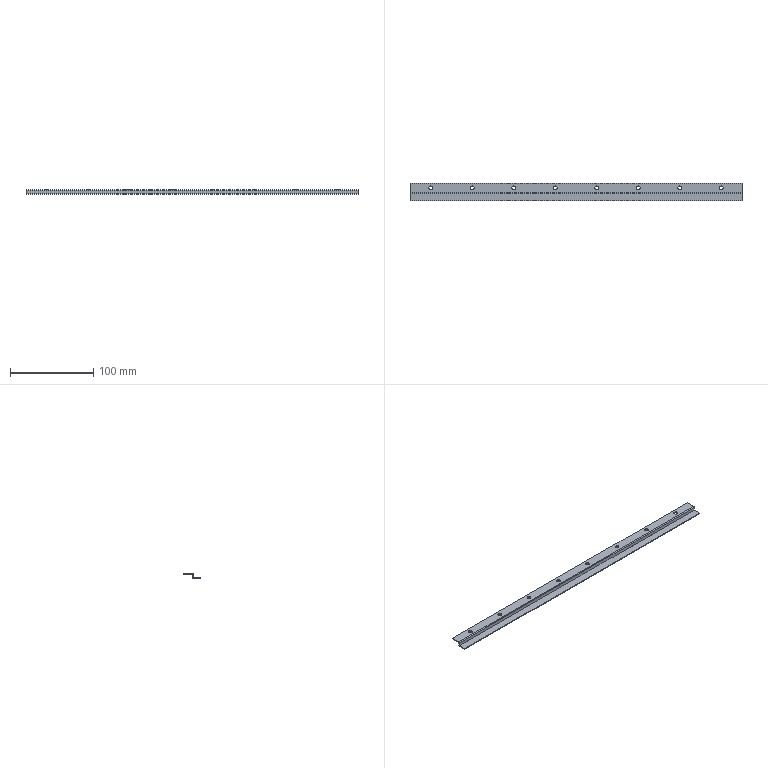Part | STEP file | 1 solid | 38 faces | box 400 x 21 x 6 mm | volume 10098 mm3 | cylinder 20 | plane 18 | commonest cylinder face diameters 4.5 x16 0.02 x2 2.02 x2